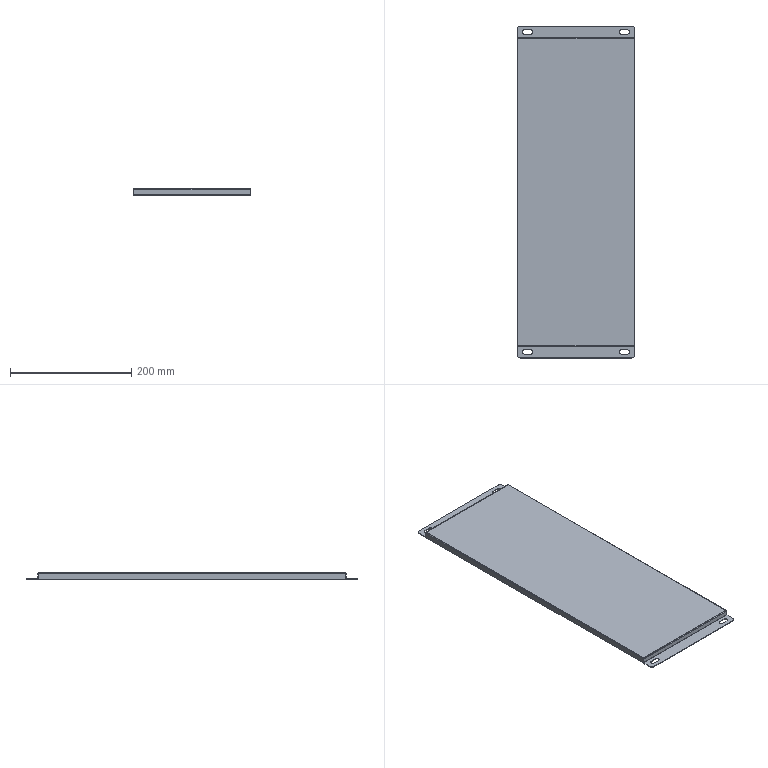Part | 1 solid | 82 faces | box 194 x 548 x 10 mm | volume 117942 mm3 | plane 54 | cylinder 28 | commonest cylinder face diameters 7 x12 0.4 x6 2.4 x6 10 x4